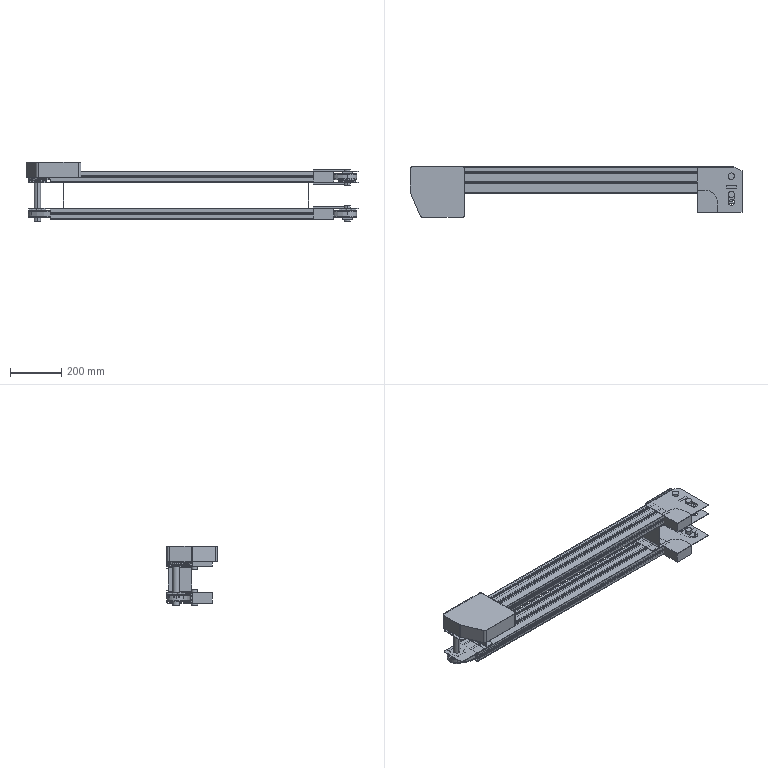Part | STEP file | TCSW62A-MD-145-1213-18-90W-3-SC-1014_no bracket 2090<machined> | 43 solids | 1656 faces | box 1300 x 197.8 x 232.2 mm | volume 4651494 mm3 | cylinder 832 | plane 824 | commonest cylinder face diameters 4.62 x240 11.91 x224 0.8 x84 25 x54 1 x46 40 x32